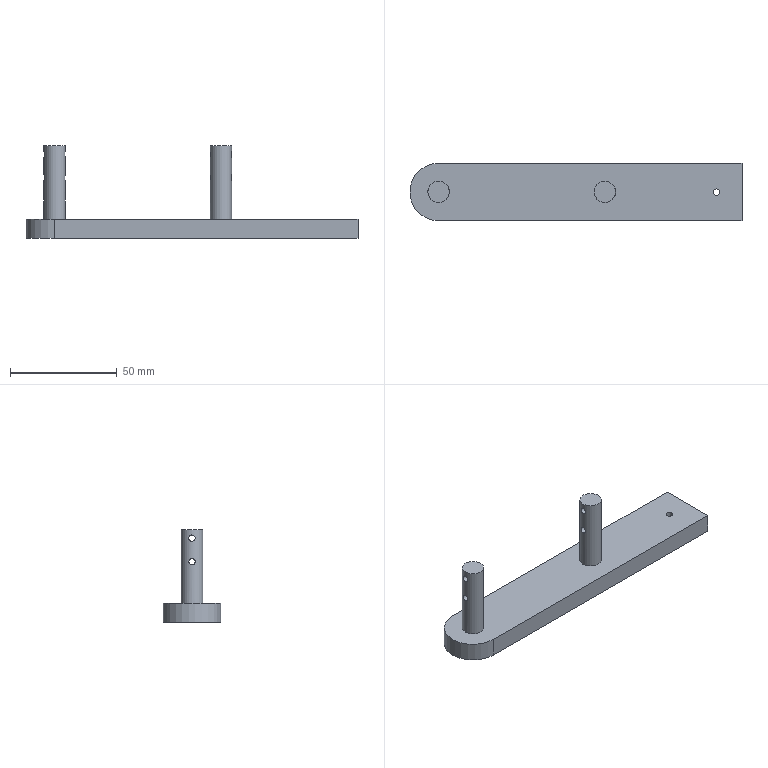Part | NX | features DATUM_CSYS 3, EXTRUDE 3, SKETCH 2, DATUM_PLANE 1 | 1 solid | 15 faces | box 155.8 x 27 x 43.5 mm | volume 42232 mm3 | cylinder 8 | plane 7 | commonest cylinder face diameters 3 x5 10 x2 27 x1
STEP:
#1=CARTESIAN_POINT('',(0.0002022,13.5,-5.5));
#2=VERTEX_POINT('',#1);
#3=CARTESIAN_POINT('',(0.0002022,-13.5,-5.5));
#4=VERTEX_POINT('',#3);
#5=CARTESIAN_POINT('',(0.0002022,-0.000000364,-5.5));
#6=DIRECTION('',(0.,0.,1.));
#7=DIRECTION('',(0.,1.,0.));
#8=AXIS2_PLACEMENT_3D('',#5,#6,#7);
#9=CIRCLE('',#8,13.5);
#10=EDGE_CURVE('',#2,#4,#9,.T.);
#11=ORIENTED_EDGE('',*,*,#10,.F.);
#12=CARTESIAN_POINT('',(0.0002022,13.5,-14.5));
#13=VERTEX_POINT('',#12);
#14=CARTESIAN_POINT('',(0.0002022,13.5,-14.5));
#15=DIRECTION('',(0.,0.,1.));
#16=VECTOR('',#15,1000.);
#17=LINE('',#14,#16);
#18=EDGE_CURVE('',#13,#2,#17,.T.);
#19=ORIENTED_EDGE('',*,*,#18,.F.);
#20=CARTESIAN_POINT('',(0.0002022,-13.5,-14.5));
#21=VERTEX_POINT('',#20);
#22=CARTESIAN_POINT('',(0.0002022,-0.000000364,-14.5));
#23=DIRECTION('',(0.,0.,1.));
#24=DIRECTION('',(0.,1.,0.));
#25=AXIS2_PLACEMENT_3D('',#22,#23,#24);
#26=CIRCLE('',#25,13.5);
#27=EDGE_CURVE('',#13,#21,#26,.T.);
#28=ORIENTED_EDGE('',*,*,#27,.T.);
#29=CARTESIAN_POINT('',(0.0002022,-13.5,-14.5));
#30=DIRECTION('',(0.,0.,1.));
#31=VECTOR('',#30,1000.);
#32=LINE('',#29,#31);
#33=EDGE_CURVE('',#21,#4,#32,.T.);
#34=ORIENTED_EDGE('',*,*,#33,.T.);
#35=EDGE_LOOP('',(#11,#19,#28,#34));
#36=FACE_BOUND('',#35,.T.);
#37=CARTESIAN_POINT('',(0.0002022,-0.000000364,-14.5));
#38=DIRECTION('',(0.,0.,1.));
#39=DIRECTION('',(1.,0.,0.));
#40=AXIS2_PLACEMENT_3D('',#37,#38,#39);
#41=CYLINDRICAL_SURFACE('',#40,13.5);
#42=ADVANCED_FACE('',(#36),#41,.T.);
#43=CARTESIAN_POINT('',(142.3,-13.5,-5.5));
#44=VERTEX_POINT('',#43);
#45=CARTESIAN_POINT('',(0.0002022,-13.5,-5.5));
#46=DIRECTION('',(1.,0.,0.));
#47=VECTOR('',#46,1000.);
#48=LINE('',#45,#47);
#49=EDGE_CURVE('',#4,#44,#48,.T.);
#50=ORIENTED_EDGE('',*,*,#49,.F.);
#51=ORIENTED_EDGE('',*,*,#33,.F.);
#52=CARTESIAN_POINT('',(142.3,-13.5,-14.5));
#53=VERTEX_POINT('',#52);
#54=CARTESIAN_POINT('',(0.0002022,-13.5,-14.5));
#55=DIRECTION('',(1.,0.,0.));
#56=VECTOR('',#55,1000.);
#57=LINE('',#54,#56);
#58=EDGE_CURVE('',#21,#53,#57,.T.);
#59=ORIENTED_EDGE('',*,*,#58,.T.);
#60=CARTESIAN_POINT('',(142.3,-13.5,-14.5));
#61=DIRECTION('',(0.,0.,1.));
#62=VECTOR('',#61,1000.);
#63=LINE('',#60,#62);
#64=EDGE_CURVE('',#53,#44,#63,.T.);
#65=ORIENTED_EDGE('',*,*,#64,.T.);
#66=EDGE_LOOP('',(#50,#51,#59,#65));
#67=FACE_BOUND('',#66,.T.);
#68=CARTESIAN_POINT('',(0.0002022,-13.5,-14.5));
#69=DIRECTION('',(0.,-1.,0.));
#70=DIRECTION('',(0.,0.,-1.));
#71=AXIS2_PLACEMENT_3D('',#68,#69,#70);
#72=PLANE('',#71);
#73=ADVANCED_FACE('',(#67),#72,.T.);
#74=CARTESIAN_POINT('',(142.3,13.5,-5.5));
#75=VERTEX_POINT('',#74);
#76=CARTESIAN_POINT('',(142.3,-13.5,-5.5));
#77=DIRECTION('',(0.,1.,0.));
#78=VECTOR('',#77,1000.);
#79=LINE('',#76,#78);
#80=EDGE_CURVE('',#44,#75,#79,.T.);
#81=ORIENTED_EDGE('',*,*,#80,.F.);
#82=ORIENTED_EDGE('',*,*,#64,.F.);
#83=CARTESIAN_POINT('',(142.3,13.5,-14.5));
#84=VERTEX_POINT('',#83);
#85=CARTESIAN_POINT('',(142.3,-13.5,-14.5));
#86=DIRECTION('',(0.,1.,0.));
#87=VECTOR('',#86,1000.);
#88=LINE('',#85,#87);
#89=EDGE_CURVE('',#53,#84,#88,.T.);
#90=ORIENTED_EDGE('',*,*,#89,.T.);
#91=CARTESIAN_POINT('',(142.3,13.5,-14.5));
#92=DIRECTION('',(0.,0.,1.));
#93=VECTOR('',#92,1000.);
#94=LINE('',#91,#93);
#95=EDGE_CURVE('',#84,#75,#94,.T.);
#96=ORIENTED_EDGE('',*,*,#95,.T.);
#97=EDGE_LOOP('',(#81,#82,#90,#96));
#98=FACE_BOUND('',#97,.T.);
#99=CARTESIAN_POINT('',(142.3,-13.5,-14.5));
#100=DIRECTION('',(1.,0.,0.));
#101=DIRECTION('',(0.,0.,-1.));
#102=AXIS2_PLACEMENT_3D('',#99,#100,#101);
#103=PLANE('',#102);
#104=ADVANCED_FACE('',(#98),#103,.T.);
#105=CARTESIAN_POINT('',(142.3,13.5,-5.5));
#106=DIRECTION('',(-1.,0.,0.));
#107=VECTOR('',#106,1000.);
#108=LINE('',#105,#107);
#109=EDGE_CURVE('',#75,#2,#108,.T.);
#110=ORIENTED_EDGE('',*,*,#109,.F.);
#111=ORIENTED_EDGE('',*,*,#95,.F.);
#112=CARTESIAN_POINT('',(142.3,13.5,-14.5));
#113=DIRECTION('',(-1.,0.,0.));
#114=VECTOR('',#113,1000.);
#115=LINE('',#112,#114);
#116=EDGE_CURVE('',#84,#13,#115,.T.);
#117=ORIENTED_EDGE('',*,*,#116,.T.);
#118=ORIENTED_EDGE('',*,*,#18,.T.);
#119=EDGE_LOOP('',(#110,#111,#117,#118));
#120=FACE_BOUND('',#119,.T.);
#121=CARTESIAN_POINT('',(142.3,13.5,-14.5));
#122=DIRECTION('',(0.,1.,0.));
#123=DIRECTION('',(0.,0.,1.));
#124=AXIS2_PLACEMENT_3D('',#121,#122,#123);
#125=PLANE('',#124);
#126=ADVANCED_FACE('',(#120),#125,.T.);
#127=CARTESIAN_POINT('',(131.82,-0.03268,-14.5));
#128=VERTEX_POINT('',#127);
#129=CARTESIAN_POINT('',(130.32,-0.03268,-14.5));
#130=DIRECTION('',(0.,0.,1.));
#131=DIRECTION('',(1.,0.,0.));
#132=AXIS2_PLACEMENT_3D('',#129,#130,#131);
#133=CIRCLE('',#132,1.5);
#134=EDGE_CURVE('',#128,#128,#133,.T.);
#135=ORIENTED_EDGE('',*,*,#134,.F.);
#136=EDGE_LOOP('',(#135));
#137=FACE_BOUND('',#136,.T.);
#138=CARTESIAN_POINT('',(131.82,-0.03268,-5.5));
#139=VERTEX_POINT('',#138);
#140=CARTESIAN_POINT('',(130.32,-0.03268,-5.5));
#141=DIRECTION('',(0.,0.,1.));
#142=DIRECTION('',(1.,0.,0.));
#143=AXIS2_PLACEMENT_3D('',#140,#141,#142);
#144=CIRCLE('',#143,1.5);
#145=EDGE_CURVE('',#139,#139,#144,.T.);
#146=ORIENTED_EDGE('',*,*,#145,.T.);
#147=EDGE_LOOP('',(#146));
#148=FACE_BOUND('',#147,.T.);
#149=CARTESIAN_POINT('',(130.32,-0.03268,-14.5));
#150=DIRECTION('',(0.,0.,1.));
#151=DIRECTION('',(1.,0.,0.));
#152=AXIS2_PLACEMENT_3D('',#149,#150,#151);
#153=CYLINDRICAL_SURFACE('',#152,1.5);
#154=ADVANCED_FACE('',(#137,#148),#153,.F.);
#155=ORIENTED_EDGE('',*,*,#27,.F.);
#156=ORIENTED_EDGE('',*,*,#116,.F.);
#157=ORIENTED_EDGE('',*,*,#89,.F.);
#158=ORIENTED_EDGE('',*,*,#58,.F.);
#159=EDGE_LOOP('',(#155,#156,#157,#158));
#160=FACE_BOUND('',#159,.T.);
#161=ORIENTED_EDGE('',*,*,#134,.T.);
#162=EDGE_LOOP('',(#161));
#163=FACE_BOUND('',#162,.T.);
#164=CARTESIAN_POINT('',(0.0002022,-0.000000364,-14.5));
#165=DIRECTION('',(0.,0.,1.));
#166=DIRECTION('',(1.,0.,0.));
#167=AXIS2_PLACEMENT_3D('',#164,#165,#166);
#168=PLANE('',#167);
#169=ADVANCED_FACE('',(#160,#163),#168,.F.);
#170=ORIENTED_EDGE('',*,*,#10,.T.);
#171=ORIENTED_EDGE('',*,*,#49,.T.);
#172=ORIENTED_EDGE('',*,*,#80,.T.);
#173=ORIENTED_EDGE('',*,*,#109,.T.);
#174=EDGE_LOOP('',(#170,#171,#172,#173));
#175=FACE_BOUND('',#174,.T.);
#176=CARTESIAN_POINT('',(5.,-0.000000364,-5.5));
#177=VERTEX_POINT('',#176);
#178=CARTESIAN_POINT('',(0.0002022,-0.000000364,-5.5));
#179=DIRECTION('',(0.,0.,1.));
#180=DIRECTION('',(1.,0.,0.));
#181=AXIS2_PLACEMENT_3D('',#178,#179,#180);
#182=CIRCLE('',#181,5.);
#183=EDGE_CURVE('',#177,#177,#182,.T.);
#184=ORIENTED_EDGE('',*,*,#183,.F.);
#185=EDGE_LOOP('',(#184));
#186=FACE_BOUND('',#185,.T.);
#187=CARTESIAN_POINT('',(83.,-0.000000364,-5.5));
#188=VERTEX_POINT('',#187);
#189=CARTESIAN_POINT('',(78.,-0.000000364,-5.5));
#190=DIRECTION('',(0.,0.,1.));
#191=DIRECTION('',(1.,0.,0.));
#192=AXIS2_PLACEMENT_3D('',#189,#190,#191);
#193=CIRCLE('',#192,5.);
#194=EDGE_CURVE('',#188,#188,#193,.T.);
#195=ORIENTED_EDGE('',*,*,#194,.F.);
#196=EDGE_LOOP('',(#195));
#197=FACE_BOUND('',#196,.T.);
#198=ORIENTED_EDGE('',*,*,#145,.F.);
#199=EDGE_LOOP('',(#198));
#200=FACE_BOUND('',#199,.T.);
#201=CARTESIAN_POINT('',(0.0002022,-0.000000364,-5.5));
#202=DIRECTION('',(0.,0.,1.));
#203=DIRECTION('',(1.,0.,0.));
#204=AXIS2_PLACEMENT_3D('',#201,#202,#203);
#205=PLANE('',#204);
#206=ADVANCED_FACE('',(#175,#186,#197,#200),#205,.T.);
#207=CARTESIAN_POINT('',(83.,-0.000000364,29.));
#208=VERTEX_POINT('',#207);
#209=CARTESIAN_POINT('',(78.,-0.000000364,29.));
#210=DIRECTION('',(0.,0.,1.));
#211=DIRECTION('',(1.,0.,0.));
#212=AXIS2_PLACEMENT_3D('',#209,#210,#211);
#213=CIRCLE('',#212,5.);
#214=EDGE_CURVE('',#208,#208,#213,.T.);
#215=ORIENTED_EDGE('',*,*,#214,.T.);
#216=EDGE_LOOP('',(#215));
#217=FACE_BOUND('',#216,.T.);
#218=CARTESIAN_POINT('',(78.,-0.000000364,29.));
#219=DIRECTION('',(0.,0.,1.));
#220=DIRECTION('',(1.,0.,0.));
#221=AXIS2_PLACEMENT_3D('',#218,#219,#220);
#222=PLANE('',#221);
#223=ADVANCED_FACE('',(#217),#222,.T.);
#224=CARTESIAN_POINT('',(73.,-0.000000364,26.5));
#225=VERTEX_POINT('',#224);
#226=CARTESIAN_POINT('',(73.113,1.176,26.175));
#227=CARTESIAN_POINT('',(72.944,-0.0001072,26.663));
#228=CARTESIAN_POINT('',(73.113,-1.176,26.174));
#229=CARTESIAN_POINT('',(73.289,-1.662,25.002));
#230=CARTESIAN_POINT('',(73.113,-1.175,23.824));
#231=CARTESIAN_POINT('',(72.944,-0.0009052,23.338));
#232=CARTESIAN_POINT('',(73.112,1.175,23.824));
#233=CARTESIAN_POINT('',(73.289,1.662,25.));
#234=CARTESIAN_POINT('',(73.113,1.176,26.175));
#235=CARTESIAN_POINT('',(72.944,-0.0001072,26.663));
#236=CARTESIAN_POINT('',(73.113,-1.176,26.174));
#237=B_SPLINE_CURVE_WITH_KNOTS('',3,(#226,#227,#228,#229,#230,#231,#232,#233,#234,#235,#236),.UNSPECIFIED.,.T.,.F.,(1,1,1,1,1,1,1,1,1,1,1,1,1,1,1),(-0.003537,-0.002358,-0.001179,0.,0.001179,0.002358,0.003537,0.004716,0.005895,0.007075,0.008254,0.009433,0.01061,0.01179,0.01297),.UNSPECIFIED.);
#238=EDGE_CURVE('',#225,#225,#237,.T.);
#239=ORIENTED_EDGE('',*,*,#238,.T.);
#240=EDGE_LOOP('',(#239));
#241=FACE_BOUND('',#240,.T.);
#242=CARTESIAN_POINT('',(83.,-0.000001765,26.5));
#243=VERTEX_POINT('',#242);
#244=CARTESIAN_POINT('',(82.888,-1.176,26.175));
#245=CARTESIAN_POINT('',(83.057,0.0001052,26.663));
#246=CARTESIAN_POINT('',(82.888,1.176,26.174));
#247=CARTESIAN_POINT('',(82.711,1.662,25.002));
#248=CARTESIAN_POINT('',(82.888,1.175,23.824));
#249=CARTESIAN_POINT('',(83.056,0.0008998,23.338));
#250=CARTESIAN_POINT('',(82.888,-1.175,23.824));
#251=CARTESIAN_POINT('',(82.711,-1.662,25.));
#252=CARTESIAN_POINT('',(82.888,-1.176,26.175));
#253=CARTESIAN_POINT('',(83.057,0.0001052,26.663));
#254=CARTESIAN_POINT('',(82.888,1.176,26.174));
#255=B_SPLINE_CURVE_WITH_KNOTS('',3,(#244,#245,#246,#247,#248,#249,#250,#251,#252,#253,#254),.UNSPECIFIED.,.T.,.F.,(1,1,1,1,1,1,1,1,1,1,1,1,1,1,1),(-0.003537,-0.002358,-0.001179,0.,0.001179,0.002358,0.003537,0.004716,0.005895,0.007075,0.008254,0.009433,0.01061,0.01179,0.01297),.UNSPECIFIED.);
#256=EDGE_CURVE('',#243,#243,#255,.T.);
#257=ORIENTED_EDGE('',*,*,#256,.T.);
#258=EDGE_LOOP('',(#257));
#259=FACE_BOUND('',#258,.T.);
#260=CARTESIAN_POINT('',(73.,-0.000000364,15.5));
#261=VERTEX_POINT('',#260);
#262=CARTESIAN_POINT('',(73.113,1.176,15.175));
#263=CARTESIAN_POINT('',(72.944,-0.0001072,15.663));
#264=CARTESIAN_POINT('',(73.113,-1.176,15.174));
#265=CARTESIAN_POINT('',(73.289,-1.662,14.002));
#266=CARTESIAN_POINT('',(73.113,-1.175,12.824));
#267=CARTESIAN_POINT('',(72.944,-0.0009052,12.338));
#268=CARTESIAN_POINT('',(73.112,1.175,12.824));
#269=CARTESIAN_POINT('',(73.289,1.662,14.));
#270=CARTESIAN_POINT('',(73.113,1.176,15.175));
#271=CARTESIAN_POINT('',(72.944,-0.0001072,15.663));
#272=CARTESIAN_POINT('',(73.113,-1.176,15.174));
#273=B_SPLINE_CURVE_WITH_KNOTS('',3,(#262,#263,#264,#265,#266,#267,#268,#269,#270,#271,#272),.UNSPECIFIED.,.T.,.F.,(1,1,1,1,1,1,1,1,1,1,1,1,1,1,1),(-0.003537,-0.002358,-0.001179,0.,0.001179,0.002358,0.003537,0.004716,0.005895,0.007075,0.008254,0.009433,0.01061,0.01179,0.01297),.UNSPECIFIED.);
#274=EDGE_CURVE('',#261,#261,#273,.T.);
#275=ORIENTED_EDGE('',*,*,#274,.T.);
#276=EDGE_LOOP('',(#275));
#277=FACE_BOUND('',#276,.T.);
#278=CARTESIAN_POINT('',(83.,-0.000001765,15.5));
#279=VERTEX_POINT('',#278);
#280=CARTESIAN_POINT('',(82.888,-1.176,15.175));
#281=CARTESIAN_POINT('',(83.057,0.0001052,15.663));
#282=CARTESIAN_POINT('',(82.888,1.176,15.174));
#283=CARTESIAN_POINT('',(82.711,1.662,14.002));
#284=CARTESIAN_POINT('',(82.888,1.175,12.824));
#285=CARTESIAN_POINT('',(83.056,0.0008998,12.338));
#286=CARTESIAN_POINT('',(82.888,-1.175,12.824));
#287=CARTESIAN_POINT('',(82.711,-1.662,14.));
#288=CARTESIAN_POINT('',(82.888,-1.176,15.175));
#289=CARTESIAN_POINT('',(83.057,0.0001052,15.663));
#290=CARTESIAN_POINT('',(82.888,1.176,15.174));
#291=B_SPLINE_CURVE_WITH_KNOTS('',3,(#280,#281,#282,#283,#284,#285,#286,#287,#288,#289,#290),.UNSPECIFIED.,.T.,.F.,(1,1,1,1,1,1,1,1,1,1,1,1,1,1,1),(-0.003537,-0.002358,-0.001179,0.,0.001179,0.002358,0.003537,0.004716,0.005895,0.007075,0.008254,0.009433,0.01061,0.01179,0.01297),.UNSPECIFIED.);
#292=EDGE_CURVE('',#279,#279,#291,.T.);
#293=ORIENTED_EDGE('',*,*,#292,.T.);
#294=EDGE_LOOP('',(#293));
#295=FACE_BOUND('',#294,.T.);
#296=ORIENTED_EDGE('',*,*,#214,.F.);
#297=EDGE_LOOP('',(#296));
#298=FACE_BOUND('',#297,.T.);
#299=ORIENTED_EDGE('',*,*,#194,.T.);
#300=EDGE_LOOP('',(#299));
#301=FACE_BOUND('',#300,.T.);
#302=CARTESIAN_POINT('',(78.,-0.000000364,29.));
#303=DIRECTION('',(0.,0.,-1.));
#304=DIRECTION('',(-1.,0.,0.));
#305=AXIS2_PLACEMENT_3D('',#302,#303,#304);
#306=CYLINDRICAL_SURFACE('',#305,5.);
#307=ADVANCED_FACE('',(#241,#259,#277,#295,#298,#301),#306,.T.);
#308=CARTESIAN_POINT('',(5.,-0.000000364,29.));
#309=VERTEX_POINT('',#308);
#310=CARTESIAN_POINT('',(0.0002022,-0.000000364,29.));
#311=DIRECTION('',(0.,0.,1.));
#312=DIRECTION('',(1.,0.,0.));
#313=AXIS2_PLACEMENT_3D('',#310,#311,#312);
#314=CIRCLE('',#313,5.);
#315=EDGE_CURVE('',#309,#309,#314,.T.);
#316=ORIENTED_EDGE('',*,*,#315,.T.);
#317=EDGE_LOOP('',(#316));
#318=FACE_BOUND('',#317,.T.);
#319=CARTESIAN_POINT('',(0.0002022,-0.000000364,29.));
#320=DIRECTION('',(0.,0.,1.));
#321=DIRECTION('',(1.,0.,0.));
#322=AXIS2_PLACEMENT_3D('',#319,#320,#321);
#323=PLANE('',#322);
#324=ADVANCED_FACE('',(#318),#323,.T.);
#325=CARTESIAN_POINT('',(-5.,-0.000000364,26.5));
#326=VERTEX_POINT('',#325);
#327=CARTESIAN_POINT('',(-4.887,1.176,26.175));
#328=CARTESIAN_POINT('',(-5.056,-0.0001072,26.663));
#329=CARTESIAN_POINT('',(-4.887,-1.176,26.174));
#330=CARTESIAN_POINT('',(-4.711,-1.662,25.002));
#331=CARTESIAN_POINT('',(-4.887,-1.175,23.824));
#332=CARTESIAN_POINT('',(-5.056,-0.0009052,23.338));
#333=CARTESIAN_POINT('',(-4.888,1.175,23.824));
#334=CARTESIAN_POINT('',(-4.711,1.662,25.));
#335=CARTESIAN_POINT('',(-4.887,1.176,26.175));
#336=CARTESIAN_POINT('',(-5.056,-0.0001072,26.663));
#337=CARTESIAN_POINT('',(-4.887,-1.176,26.174));
#338=B_SPLINE_CURVE_WITH_KNOTS('',3,(#327,#328,#329,#330,#331,#332,#333,#334,#335,#336,#337),.UNSPECIFIED.,.T.,.F.,(1,1,1,1,1,1,1,1,1,1,1,1,1,1,1),(-0.003537,-0.002358,-0.001179,0.,0.001179,0.002358,0.003537,0.004716,0.005895,0.007075,0.008254,0.009433,0.01061,0.01179,0.01297),.UNSPECIFIED.);
#339=EDGE_CURVE('',#326,#326,#338,.T.);
#340=ORIENTED_EDGE('',*,*,#339,.T.);
#341=EDGE_LOOP('',(#340));
#342=FACE_BOUND('',#341,.T.);
#343=CARTESIAN_POINT('',(5.,-0.000001765,26.5));
#344=VERTEX_POINT('',#343);
#345=CARTESIAN_POINT('',(4.888,-1.176,26.175));
#346=CARTESIAN_POINT('',(5.057,0.0001052,26.663));
#347=CARTESIAN_POINT('',(4.888,1.176,26.174));
#348=CARTESIAN_POINT('',(4.711,1.662,25.002));
#349=CARTESIAN_POINT('',(4.888,1.175,23.824));
#350=CARTESIAN_POINT('',(5.056,0.0008998,23.338));
#351=CARTESIAN_POINT('',(4.888,-1.175,23.824));
#352=CARTESIAN_POINT('',(4.711,-1.662,25.));
#353=CARTESIAN_POINT('',(4.888,-1.176,26.175));
#354=CARTESIAN_POINT('',(5.057,0.0001052,26.663));
#355=CARTESIAN_POINT('',(4.888,1.176,26.174));
#356=B_SPLINE_CURVE_WITH_KNOTS('',3,(#345,#346,#347,#348,#349,#350,#351,#352,#353,#354,#355),.UNSPECIFIED.,.T.,.F.,(1,1,1,1,1,1,1,1,1,1,1,1,1,1,1),(-0.003537,-0.002358,-0.001179,0.,0.001179,0.002358,0.003537,0.004716,0.005895,0.007075,0.008254,0.009433,0.01061,0.01179,0.01297),.UNSPECIFIED.);
#357=EDGE_CURVE('',#344,#344,#356,.T.);
#358=ORIENTED_EDGE('',*,*,#357,.T.);
#359=EDGE_LOOP('',(#358));
#360=FACE_BOUND('',#359,.T.);
#361=CARTESIAN_POINT('',(-5.,-0.000000364,15.5));
#362=VERTEX_POINT('',#361);
#363=CARTESIAN_POINT('',(-4.887,1.176,15.175));
#364=CARTESIAN_POINT('',(-5.056,-0.0001072,15.663));
#365=CARTESIAN_POINT('',(-4.887,-1.176,15.174));
#366=CARTESIAN_POINT('',(-4.711,-1.662,14.002));
#367=CARTESIAN_POINT('',(-4.887,-1.175,12.824));
#368=CARTESIAN_POINT('',(-5.056,-0.0009052,12.338));
#369=CARTESIAN_POINT('',(-4.888,1.175,12.824));
#370=CARTESIAN_POINT('',(-4.711,1.662,14.));
#371=CARTESIAN_POINT('',(-4.887,1.176,15.175));
#372=CARTESIAN_POINT('',(-5.056,-0.0001072,15.663));
#373=CARTESIAN_POINT('',(-4.887,-1.176,15.174));
#374=B_SPLINE_CURVE_WITH_KNOTS('',3,(#363,#364,#365,#366,#367,#368,#369,#370,#371,#372,#373),.UNSPECIFIED.,.T.,.F.,(1,1,1,1,1,1,1,1,1,1,1,1,1,1,1),(-0.003537,-0.002358,-0.001179,0.,0.001179,0.002358,0.003537,0.004716,0.005895,0.007075,0.008254,0.009433,0.01061,0.01179,0.01297),.UNSPECIFIED.);
#375=EDGE_CURVE('',#362,#362,#374,.T.);
#376=ORIENTED_EDGE('',*,*,#375,.T.);
#377=EDGE_LOOP('',(#376));
#378=FACE_BOUND('',#377,.T.);
#379=CARTESIAN_POINT('',(5.,-0.000001765,15.5));
#380=VERTEX_POINT('',#379);
#381=CARTESIAN_POINT('',(4.888,-1.176,15.175));
#382=CARTESIAN_POINT('',(5.057,0.0001052,15.663));
#383=CARTESIAN_POINT('',(4.888,1.176,15.174));
#384=CARTESIAN_POINT('',(4.711,1.662,14.002));
#385=CARTESIAN_POINT('',(4.888,1.175,12.824));
#386=CARTESIAN_POINT('',(5.056,0.0008998,12.338));
#387=CARTESIAN_POINT('',(4.888,-1.175,12.824));
#388=CARTESIAN_POINT('',(4.711,-1.662,14.));
#389=CARTESIAN_POINT('',(4.888,-1.176,15.175));
#390=CARTESIAN_POINT('',(5.057,0.0001052,15.663));
#391=CARTESIAN_POINT('',(4.888,1.176,15.174));
#392=B_SPLINE_CURVE_WITH_KNOTS('',3,(#381,#382,#383,#384,#385,#386,#387,#388,#389,#390,#391),.UNSPECIFIED.,.T.,.F.,(1,1,1,1,1,1,1,1,1,1,1,1,1,1,1),(-0.003537,-0.002358,-0.001179,0.,0.001179,0.002358,0.003537,0.004716,0.005895,0.007075,0.008254,0.009433,0.01061,0.01179,0.01297),.UNSPECIFIED.);
#393=EDGE_CURVE('',#380,#380,#392,.T.);
#394=ORIENTED_EDGE('',*,*,#393,.T.);
#395=EDGE_LOOP('',(#394));
#396=FACE_BOUND('',#395,.T.);
#397=ORIENTED_EDGE('',*,*,#315,.F.);
#398=EDGE_LOOP('',(#397));
#399=FACE_BOUND('',#398,.T.);
#400=ORIENTED_EDGE('',*,*,#183,.T.);
#401=EDGE_LOOP('',(#400));
#402=FACE_BOUND('',#401,.T.);
#403=CARTESIAN_POINT('',(0.0002022,-0.000000364,29.));
#404=DIRECTION('',(0.,0.,-1.));
#405=DIRECTION('',(-1.,0.,0.));
#406=AXIS2_PLACEMENT_3D('',#403,#404,#405);
#407=CYLINDRICAL_SURFACE('',#406,5.);
#408=ADVANCED_FACE('',(#342,#360,#378,#396,#399,#402),#407,.T.);
#409=ORIENTED_EDGE('',*,*,#393,.F.);
#410=EDGE_LOOP('',(#409));
#411=FACE_BOUND('',#410,.T.);
#412=ORIENTED_EDGE('',*,*,#375,.F.);
#413=EDGE_LOOP('',(#412));
#414=FACE_BOUND('',#413,.T.);
#415=CARTESIAN_POINT('',(113.,-0.000001765,14.));
#416=DIRECTION('',(-1.,0.,0.));
#417=DIRECTION('',(0.,0.,1.));
#418=AXIS2_PLACEMENT_3D('',#415,#416,#417);
#419=CYLINDRICAL_SURFACE('',#418,1.5);
#420=ADVANCED_FACE('',(#411,#414),#419,.F.);
#421=ORIENTED_EDGE('',*,*,#292,.F.);
#422=EDGE_LOOP('',(#421));
#423=FACE_BOUND('',#422,.T.);
#424=ORIENTED_EDGE('',*,*,#274,.F.);
#425=EDGE_LOOP('',(#424));
#426=FACE_BOUND('',#425,.T.);
#427=CARTESIAN_POINT('',(113.,-0.000001765,14.));
#428=DIRECTION('',(-1.,0.,0.));
#429=DIRECTION('',(0.,0.,1.));
#430=AXIS2_PLACEMENT_3D('',#427,#428,#429);
#431=CYLINDRICAL_SURFACE('',#430,1.5);
#432=ADVANCED_FACE('',(#423,#426),#431,.F.);
#433=ORIENTED_EDGE('',*,*,#357,.F.);
#434=EDGE_LOOP('',(#433));
#435=FACE_BOUND('',#434,.T.);
#436=ORIENTED_EDGE('',*,*,#339,.F.);
#437=EDGE_LOOP('',(#436));
#438=FACE_BOUND('',#437,.T.);
#439=CARTESIAN_POINT('',(113.,-0.000001765,25.));
#440=DIRECTION('',(-1.,0.,0.));
#441=DIRECTION('',(0.,0.,1.));
#442=AXIS2_PLACEMENT_3D('',#439,#440,#441);
#443=CYLINDRICAL_SURFACE('',#442,1.5);
#444=ADVANCED_FACE('',(#435,#438),#443,.F.);
#445=ORIENTED_EDGE('',*,*,#256,.F.);
#446=EDGE_LOOP('',(#445));
#447=FACE_BOUND('',#446,.T.);
#448=ORIENTED_EDGE('',*,*,#238,.F.);
#449=EDGE_LOOP('',(#448));
#450=FACE_BOUND('',#449,.T.);
#451=CARTESIAN_POINT('',(113.,-0.000001765,25.));
#452=DIRECTION('',(-1.,0.,0.));
#453=DIRECTION('',(0.,0.,1.));
#454=AXIS2_PLACEMENT_3D('',#451,#452,#453);
#455=CYLINDRICAL_SURFACE('',#454,1.5);
#456=ADVANCED_FACE('',(#447,#450),#455,.F.);
#457=CLOSED_SHELL('',(#42,#73,#104,#126,#154,#169,#206,#223,#307,#324,#408,#420,#432,#444,#456));
#458=MANIFOLD_SOLID_BREP('',#457);
#459=(LENGTH_UNIT()NAMED_UNIT(*)SI_UNIT(.MILLI.,.METRE.));
#460=UNCERTAINTY_MEASURE_WITH_UNIT(LENGTH_MEASURE(0.0508),#459,'','');
#461=(NAMED_UNIT(*)PLANE_ANGLE_UNIT()SI_UNIT($,.RADIAN.));
#462=(NAMED_UNIT(*)SI_UNIT($,.STERADIAN.)SOLID_ANGLE_UNIT());
#463=(GEOMETRIC_REPRESENTATION_CONTEXT(3)GLOBAL_UNCERTAINTY_ASSIGNED_CONTEXT((#460))GLOBAL_UNIT_ASSIGNED_CONTEXT((#459,#461,#462))REPRESENTATION_CONTEXT('',''));
#464=ADVANCED_BREP_SHAPE_REPRESENTATION('',(#458),#463);